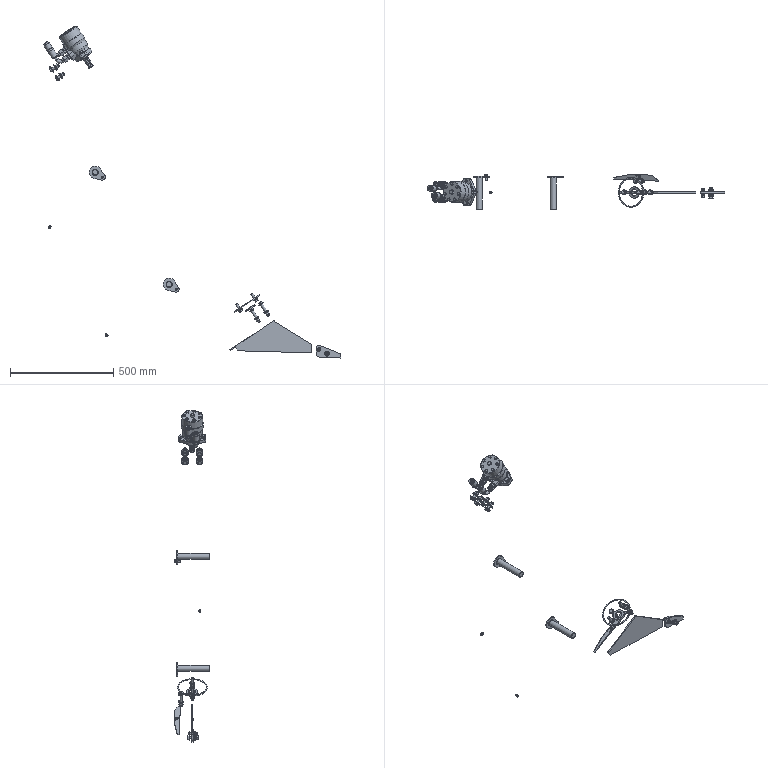Part | STEP file | COMPOUND | 76 solids | 1195 faces | box 1441 x 170.85 x 1608 mm | volume 1889259 mm3 | plane 678 | cylinder 236 | cone 163 | other 82 | torus 28 | spline 6 | sphere 2 | commonest cylinder face diameters 13 x21 10 x17 12 x16 20 x11 24 x9 30 x9